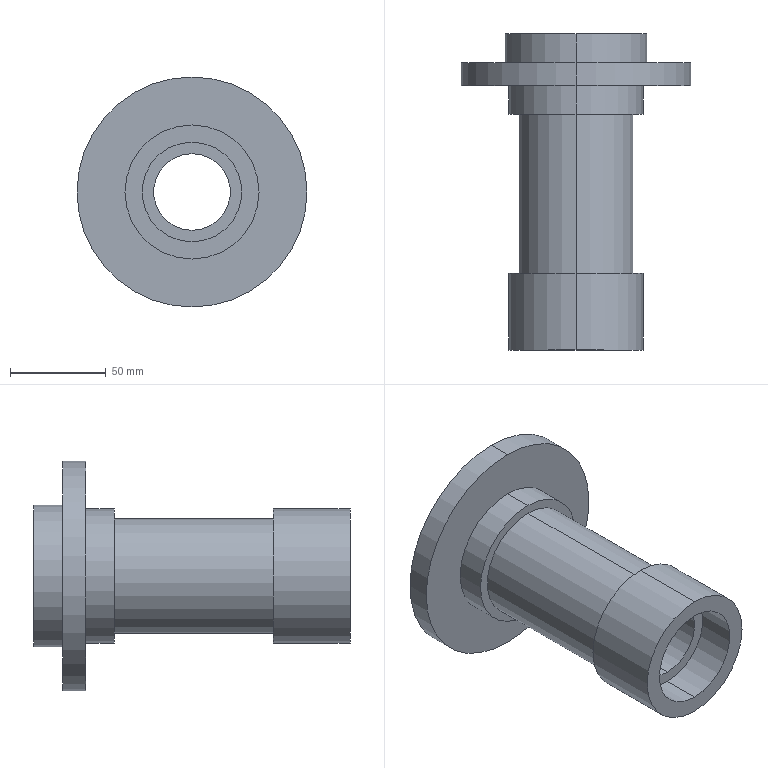Part | SolidWorks | features Revolution 1 | 1 solid | 24 faces | box 120 x 165 x 120 mm | volume 395872 mm3 | cylinder 16 | plane 8 | commonest cylinder face diameters 52 x4 70 x4 40 x2 60 x2 74 x2 120 x2
STEP:
#1=CARTESIAN_POINT('',(521.231,804.896,-470.693));
#2=VERTEX_POINT('',#1);
#3=CARTESIAN_POINT('',(521.231,804.896,-410.693));
#4=VERTEX_POINT('',#3);
#5=CARTESIAN_POINT('',(521.231,804.896,-440.693));
#6=DIRECTION('',(0.,-1.,0.));
#7=DIRECTION('',(0.,0.,-1.));
#8=AXIS2_PLACEMENT_3D('',#5,#6,#7);
#9=CIRCLE('',#8,30.);
#10=EDGE_CURVE('',#2,#4,#9,.T.);
#11=ORIENTED_EDGE('',*,*,#10,.T.);
#12=CARTESIAN_POINT('',(521.231,721.896,-410.693));
#13=VERTEX_POINT('',#12);
#14=CARTESIAN_POINT('',(521.231,846.896,-410.693));
#15=DIRECTION('',(0.,-1.,0.));
#16=VECTOR('',#15,1000.);
#17=LINE('',#14,#16);
#18=EDGE_CURVE('',#4,#13,#17,.T.);
#19=ORIENTED_EDGE('',*,*,#18,.T.);
#20=CARTESIAN_POINT('',(521.231,721.896,-470.693));
#21=VERTEX_POINT('',#20);
#22=CARTESIAN_POINT('',(521.231,721.896,-440.693));
#23=DIRECTION('',(0.,-1.,0.));
#24=DIRECTION('',(0.,0.,-1.));
#25=AXIS2_PLACEMENT_3D('',#22,#23,#24);
#26=CIRCLE('',#25,30.);
#27=EDGE_CURVE('',#21,#13,#26,.T.);
#28=ORIENTED_EDGE('',*,*,#27,.F.);
#29=CARTESIAN_POINT('',(521.231,846.896,-470.693));
#30=DIRECTION('',(0.,-1.,0.));
#31=VECTOR('',#30,1000.);
#32=LINE('',#29,#31);
#33=EDGE_CURVE('',#2,#21,#32,.T.);
#34=ORIENTED_EDGE('',*,*,#33,.F.);
#35=EDGE_LOOP('',(#11,#19,#28,#34));
#36=FACE_OUTER_BOUND('',#35,.T.);
#37=CARTESIAN_POINT('',(521.231,846.896,-440.693));
#38=DIRECTION('',(0.,-1.,0.));
#39=DIRECTION('',(0.,0.,-1.));
#40=AXIS2_PLACEMENT_3D('',#37,#38,#39);
#41=CYLINDRICAL_SURFACE('',#40,30.);
#42=ADVANCED_FACE('',(#36),#41,.T.);
#43=CARTESIAN_POINT('',(521.231,819.896,-475.693));
#44=VERTEX_POINT('',#43);
#45=CARTESIAN_POINT('',(521.231,819.896,-405.693));
#46=VERTEX_POINT('',#45);
#47=CARTESIAN_POINT('',(521.231,819.896,-440.693));
#48=DIRECTION('',(0.,-1.,0.));
#49=DIRECTION('',(0.,0.,-1.));
#50=AXIS2_PLACEMENT_3D('',#47,#48,#49);
#51=CIRCLE('',#50,35.);
#52=EDGE_CURVE('',#44,#46,#51,.T.);
#53=ORIENTED_EDGE('',*,*,#52,.T.);
#54=CARTESIAN_POINT('',(521.231,804.896,-405.693));
#55=VERTEX_POINT('',#54);
#56=CARTESIAN_POINT('',(521.231,846.896,-405.693));
#57=DIRECTION('',(0.,-1.,0.));
#58=VECTOR('',#57,1000.);
#59=LINE('',#56,#58);
#60=EDGE_CURVE('',#46,#55,#59,.T.);
#61=ORIENTED_EDGE('',*,*,#60,.T.);
#62=CARTESIAN_POINT('',(521.231,804.896,-475.693));
#63=VERTEX_POINT('',#62);
#64=CARTESIAN_POINT('',(521.231,804.896,-440.693));
#65=DIRECTION('',(0.,-1.,0.));
#66=DIRECTION('',(0.,0.,-1.));
#67=AXIS2_PLACEMENT_3D('',#64,#65,#66);
#68=CIRCLE('',#67,35.);
#69=EDGE_CURVE('',#63,#55,#68,.T.);
#70=ORIENTED_EDGE('',*,*,#69,.F.);
#71=CARTESIAN_POINT('',(521.231,846.896,-475.693));
#72=DIRECTION('',(0.,-1.,0.));
#73=VECTOR('',#72,1000.);
#74=LINE('',#71,#73);
#75=EDGE_CURVE('',#44,#63,#74,.T.);
#76=ORIENTED_EDGE('',*,*,#75,.F.);
#77=EDGE_LOOP('',(#53,#61,#70,#76));
#78=FACE_OUTER_BOUND('',#77,.T.);
#79=CARTESIAN_POINT('',(521.231,846.896,-440.693));
#80=DIRECTION('',(0.,-1.,0.));
#81=DIRECTION('',(0.,0.,-1.));
#82=AXIS2_PLACEMENT_3D('',#79,#80,#81);
#83=CYLINDRICAL_SURFACE('',#82,35.);
#84=ADVANCED_FACE('',(#78),#83,.T.);
#85=CARTESIAN_POINT('',(521.231,831.896,-500.693));
#86=VERTEX_POINT('',#85);
#87=CARTESIAN_POINT('',(521.231,831.896,-380.693));
#88=VERTEX_POINT('',#87);
#89=CARTESIAN_POINT('',(521.231,831.896,-440.693));
#90=DIRECTION('',(0.,-1.,0.));
#91=DIRECTION('',(0.,0.,-1.));
#92=AXIS2_PLACEMENT_3D('',#89,#90,#91);
#93=CIRCLE('',#92,60.);
#94=EDGE_CURVE('',#86,#88,#93,.T.);
#95=ORIENTED_EDGE('',*,*,#94,.T.);
#96=CARTESIAN_POINT('',(521.231,819.896,-380.693));
#97=VERTEX_POINT('',#96);
#98=CARTESIAN_POINT('',(521.231,846.896,-380.693));
#99=DIRECTION('',(0.,-1.,0.));
#100=VECTOR('',#99,1000.);
#101=LINE('',#98,#100);
#102=EDGE_CURVE('',#88,#97,#101,.T.);
#103=ORIENTED_EDGE('',*,*,#102,.T.);
#104=CARTESIAN_POINT('',(521.231,819.896,-500.693));
#105=VERTEX_POINT('',#104);
#106=CARTESIAN_POINT('',(521.231,819.896,-440.693));
#107=DIRECTION('',(0.,-1.,0.));
#108=DIRECTION('',(0.,0.,-1.));
#109=AXIS2_PLACEMENT_3D('',#106,#107,#108);
#110=CIRCLE('',#109,60.);
#111=EDGE_CURVE('',#105,#97,#110,.T.);
#112=ORIENTED_EDGE('',*,*,#111,.F.);
#113=CARTESIAN_POINT('',(521.231,846.896,-500.693));
#114=DIRECTION('',(0.,-1.,0.));
#115=VECTOR('',#114,1000.);
#116=LINE('',#113,#115);
#117=EDGE_CURVE('',#86,#105,#116,.T.);
#118=ORIENTED_EDGE('',*,*,#117,.F.);
#119=EDGE_LOOP('',(#95,#103,#112,#118));
#120=FACE_OUTER_BOUND('',#119,.T.);
#121=CARTESIAN_POINT('',(521.231,846.896,-440.693));
#122=DIRECTION('',(0.,-1.,0.));
#123=DIRECTION('',(0.,0.,-1.));
#124=AXIS2_PLACEMENT_3D('',#121,#122,#123);
#125=CYLINDRICAL_SURFACE('',#124,60.);
#126=ADVANCED_FACE('',(#120),#125,.T.);
#127=CARTESIAN_POINT('',(521.231,846.896,-477.693));
#128=VERTEX_POINT('',#127);
#129=CARTESIAN_POINT('',(521.231,846.896,-403.693));
#130=VERTEX_POINT('',#129);
#131=CARTESIAN_POINT('',(521.231,846.896,-440.693));
#132=DIRECTION('',(0.,-1.,0.));
#133=DIRECTION('',(0.,0.,-1.));
#134=AXIS2_PLACEMENT_3D('',#131,#132,#133);
#135=CIRCLE('',#134,37.);
#136=EDGE_CURVE('',#128,#130,#135,.T.);
#137=ORIENTED_EDGE('',*,*,#136,.T.);
#138=CARTESIAN_POINT('',(521.231,831.896,-403.693));
#139=VERTEX_POINT('',#138);
#140=CARTESIAN_POINT('',(521.231,846.896,-403.693));
#141=DIRECTION('',(0.,-1.,0.));
#142=VECTOR('',#141,1000.);
#143=LINE('',#140,#142);
#144=EDGE_CURVE('',#130,#139,#143,.T.);
#145=ORIENTED_EDGE('',*,*,#144,.T.);
#146=CARTESIAN_POINT('',(521.231,831.896,-477.693));
#147=VERTEX_POINT('',#146);
#148=CARTESIAN_POINT('',(521.231,831.896,-440.693));
#149=DIRECTION('',(0.,-1.,0.));
#150=DIRECTION('',(0.,0.,-1.));
#151=AXIS2_PLACEMENT_3D('',#148,#149,#150);
#152=CIRCLE('',#151,37.);
#153=EDGE_CURVE('',#147,#139,#152,.T.);
#154=ORIENTED_EDGE('',*,*,#153,.F.);
#155=CARTESIAN_POINT('',(521.231,846.896,-477.693));
#156=DIRECTION('',(0.,-1.,0.));
#157=VECTOR('',#156,1000.);
#158=LINE('',#155,#157);
#159=EDGE_CURVE('',#128,#147,#158,.T.);
#160=ORIENTED_EDGE('',*,*,#159,.F.);
#161=EDGE_LOOP('',(#137,#145,#154,#160));
#162=FACE_OUTER_BOUND('',#161,.T.);
#163=CARTESIAN_POINT('',(521.231,846.896,-440.693));
#164=DIRECTION('',(0.,-1.,0.));
#165=DIRECTION('',(0.,0.,-1.));
#166=AXIS2_PLACEMENT_3D('',#163,#164,#165);
#167=CYLINDRICAL_SURFACE('',#166,37.);
#168=ADVANCED_FACE('',(#162),#167,.T.);
#169=CARTESIAN_POINT('',(521.231,846.896,-414.693));
#170=VERTEX_POINT('',#169);
#171=CARTESIAN_POINT('',(521.231,846.896,-466.693));
#172=VERTEX_POINT('',#171);
#173=CARTESIAN_POINT('',(521.231,846.896,-440.693));
#174=DIRECTION('',(0.,-1.,0.));
#175=DIRECTION('',(0.,0.,-1.));
#176=AXIS2_PLACEMENT_3D('',#173,#174,#175);
#177=CIRCLE('',#176,26.);
#178=EDGE_CURVE('',#170,#172,#177,.T.);
#179=ORIENTED_EDGE('',*,*,#178,.F.);
#180=CARTESIAN_POINT('',(521.231,816.896,-414.693));
#181=VERTEX_POINT('',#180);
#182=CARTESIAN_POINT('',(521.231,846.896,-414.693));
#183=DIRECTION('',(0.,-1.,0.));
#184=VECTOR('',#183,1000.);
#185=LINE('',#182,#184);
#186=EDGE_CURVE('',#170,#181,#185,.T.);
#187=ORIENTED_EDGE('',*,*,#186,.T.);
#188=CARTESIAN_POINT('',(521.231,816.896,-466.693));
#189=VERTEX_POINT('',#188);
#190=CARTESIAN_POINT('',(521.231,816.896,-440.693));
#191=DIRECTION('',(0.,-1.,0.));
#192=DIRECTION('',(0.,0.,-1.));
#193=AXIS2_PLACEMENT_3D('',#190,#191,#192);
#194=CIRCLE('',#193,26.);
#195=EDGE_CURVE('',#181,#189,#194,.T.);
#196=ORIENTED_EDGE('',*,*,#195,.T.);
#197=CARTESIAN_POINT('',(521.231,846.896,-466.693));
#198=DIRECTION('',(0.,-1.,0.));
#199=VECTOR('',#198,1000.);
#200=LINE('',#197,#199);
#201=EDGE_CURVE('',#172,#189,#200,.T.);
#202=ORIENTED_EDGE('',*,*,#201,.F.);
#203=EDGE_LOOP('',(#179,#187,#196,#202));
#204=FACE_OUTER_BOUND('',#203,.T.);
#205=CARTESIAN_POINT('',(521.231,846.896,-440.693));
#206=DIRECTION('',(0.,-1.,0.));
#207=DIRECTION('',(0.,0.,-1.));
#208=AXIS2_PLACEMENT_3D('',#205,#206,#207);
#209=CYLINDRICAL_SURFACE('',#208,26.);
#210=ADVANCED_FACE('',(#204),#209,.F.);
#211=CARTESIAN_POINT('',(521.231,816.896,-420.693));
#212=VERTEX_POINT('',#211);
#213=CARTESIAN_POINT('',(521.231,816.896,-460.693));
#214=VERTEX_POINT('',#213);
#215=CARTESIAN_POINT('',(521.231,816.896,-440.693));
#216=DIRECTION('',(0.,-1.,0.));
#217=DIRECTION('',(0.,0.,-1.));
#218=AXIS2_PLACEMENT_3D('',#215,#216,#217);
#219=CIRCLE('',#218,20.);
#220=EDGE_CURVE('',#212,#214,#219,.T.);
#221=ORIENTED_EDGE('',*,*,#220,.F.);
#222=CARTESIAN_POINT('',(521.231,701.896,-420.693));
#223=VERTEX_POINT('',#222);
#224=CARTESIAN_POINT('',(521.231,846.896,-420.693));
#225=DIRECTION('',(0.,-1.,0.));
#226=VECTOR('',#225,1000.);
#227=LINE('',#224,#226);
#228=EDGE_CURVE('',#212,#223,#227,.T.);
#229=ORIENTED_EDGE('',*,*,#228,.T.);
#230=CARTESIAN_POINT('',(521.231,701.896,-460.693));
#231=VERTEX_POINT('',#230);
#232=CARTESIAN_POINT('',(521.231,701.896,-440.693));
#233=DIRECTION('',(0.,-1.,0.));
#234=DIRECTION('',(0.,0.,-1.));
#235=AXIS2_PLACEMENT_3D('',#232,#233,#234);
#236=CIRCLE('',#235,20.);
#237=EDGE_CURVE('',#223,#231,#236,.T.);
#238=ORIENTED_EDGE('',*,*,#237,.T.);
#239=CARTESIAN_POINT('',(521.231,846.896,-460.693));
#240=DIRECTION('',(0.,-1.,0.));
#241=VECTOR('',#240,1000.);
#242=LINE('',#239,#241);
#243=EDGE_CURVE('',#214,#231,#242,.T.);
#244=ORIENTED_EDGE('',*,*,#243,.F.);
#245=EDGE_LOOP('',(#221,#229,#238,#244));
#246=FACE_OUTER_BOUND('',#245,.T.);
#247=CARTESIAN_POINT('',(521.231,846.896,-440.693));
#248=DIRECTION('',(0.,-1.,0.));
#249=DIRECTION('',(0.,0.,-1.));
#250=AXIS2_PLACEMENT_3D('',#247,#248,#249);
#251=CYLINDRICAL_SURFACE('',#250,20.);
#252=ADVANCED_FACE('',(#246),#251,.F.);
#253=CARTESIAN_POINT('',(521.231,701.896,-414.693));
#254=VERTEX_POINT('',#253);
#255=CARTESIAN_POINT('',(521.231,701.896,-466.693));
#256=VERTEX_POINT('',#255);
#257=CARTESIAN_POINT('',(521.231,701.896,-440.693));
#258=DIRECTION('',(0.,-1.,0.));
#259=DIRECTION('',(0.,0.,-1.));
#260=AXIS2_PLACEMENT_3D('',#257,#258,#259);
#261=CIRCLE('',#260,26.);
#262=EDGE_CURVE('',#254,#256,#261,.T.);
#263=ORIENTED_EDGE('',*,*,#262,.F.);
#264=CARTESIAN_POINT('',(521.231,681.896,-414.693));
#265=VERTEX_POINT('',#264);
#266=CARTESIAN_POINT('',(521.231,846.896,-414.693));
#267=DIRECTION('',(0.,-1.,0.));
#268=VECTOR('',#267,1000.);
#269=LINE('',#266,#268);
#270=EDGE_CURVE('',#254,#265,#269,.T.);
#271=ORIENTED_EDGE('',*,*,#270,.T.);
#272=CARTESIAN_POINT('',(521.231,681.896,-466.693));
#273=VERTEX_POINT('',#272);
#274=CARTESIAN_POINT('',(521.231,681.896,-440.693));
#275=DIRECTION('',(0.,-1.,0.));
#276=DIRECTION('',(0.,0.,-1.));
#277=AXIS2_PLACEMENT_3D('',#274,#275,#276);
#278=CIRCLE('',#277,26.);
#279=EDGE_CURVE('',#265,#273,#278,.T.);
#280=ORIENTED_EDGE('',*,*,#279,.T.);
#281=CARTESIAN_POINT('',(521.231,846.896,-466.693));
#282=DIRECTION('',(0.,-1.,0.));
#283=VECTOR('',#282,1000.);
#284=LINE('',#281,#283);
#285=EDGE_CURVE('',#256,#273,#284,.T.);
#286=ORIENTED_EDGE('',*,*,#285,.F.);
#287=EDGE_LOOP('',(#263,#271,#280,#286));
#288=FACE_OUTER_BOUND('',#287,.T.);
#289=CARTESIAN_POINT('',(521.231,846.896,-440.693));
#290=DIRECTION('',(0.,-1.,0.));
#291=DIRECTION('',(0.,0.,-1.));
#292=AXIS2_PLACEMENT_3D('',#289,#290,#291);
#293=CYLINDRICAL_SURFACE('',#292,26.);
#294=ADVANCED_FACE('',(#288),#293,.F.);
#295=CARTESIAN_POINT('',(521.231,721.896,-475.693));
#296=VERTEX_POINT('',#295);
#297=CARTESIAN_POINT('',(521.231,721.896,-405.693));
#298=VERTEX_POINT('',#297);
#299=CARTESIAN_POINT('',(521.231,721.896,-440.693));
#300=DIRECTION('',(0.,-1.,0.));
#301=DIRECTION('',(0.,0.,-1.));
#302=AXIS2_PLACEMENT_3D('',#299,#300,#301);
#303=CIRCLE('',#302,35.);
#304=EDGE_CURVE('',#296,#298,#303,.T.);
#305=ORIENTED_EDGE('',*,*,#304,.T.);
#306=CARTESIAN_POINT('',(521.231,681.896,-405.693));
#307=VERTEX_POINT('',#306);
#308=CARTESIAN_POINT('',(521.231,846.896,-405.693));
#309=DIRECTION('',(0.,-1.,0.));
#310=VECTOR('',#309,1000.);
#311=LINE('',#308,#310);
#312=EDGE_CURVE('',#298,#307,#311,.T.);
#313=ORIENTED_EDGE('',*,*,#312,.T.);
#314=CARTESIAN_POINT('',(521.231,681.896,-475.693));
#315=VERTEX_POINT('',#314);
#316=CARTESIAN_POINT('',(521.231,681.896,-440.693));
#317=DIRECTION('',(0.,-1.,0.));
#318=DIRECTION('',(0.,0.,-1.));
#319=AXIS2_PLACEMENT_3D('',#316,#317,#318);
#320=CIRCLE('',#319,35.);
#321=EDGE_CURVE('',#315,#307,#320,.T.);
#322=ORIENTED_EDGE('',*,*,#321,.F.);
#323=CARTESIAN_POINT('',(521.231,846.896,-475.693));
#324=DIRECTION('',(0.,-1.,0.));
#325=VECTOR('',#324,1000.);
#326=LINE('',#323,#325);
#327=EDGE_CURVE('',#296,#315,#326,.T.);
#328=ORIENTED_EDGE('',*,*,#327,.F.);
#329=EDGE_LOOP('',(#305,#313,#322,#328));
#330=FACE_OUTER_BOUND('',#329,.T.);
#331=CARTESIAN_POINT('',(521.231,846.896,-440.693));
#332=DIRECTION('',(0.,-1.,0.));
#333=DIRECTION('',(0.,0.,-1.));
#334=AXIS2_PLACEMENT_3D('',#331,#332,#333);
#335=CYLINDRICAL_SURFACE('',#334,35.);
#336=ADVANCED_FACE('',(#330),#335,.T.);
#337=ORIENTED_EDGE('',*,*,#27,.T.);
#338=CARTESIAN_POINT('',(521.231,721.896,-440.693));
#339=DIRECTION('',(0.,-1.,0.));
#340=DIRECTION('',(0.,0.,-1.));
#341=AXIS2_PLACEMENT_3D('',#338,#339,#340);
#342=CIRCLE('',#341,30.);
#343=EDGE_CURVE('',#13,#21,#342,.T.);
#344=ORIENTED_EDGE('',*,*,#343,.T.);
#345=EDGE_LOOP('',(#337,#344));
#346=FACE_BOUND('',#345,.T.);
#347=ORIENTED_EDGE('',*,*,#304,.F.);
#348=CARTESIAN_POINT('',(521.231,721.896,-440.693));
#349=DIRECTION('',(0.,-1.,0.));
#350=DIRECTION('',(0.,0.,-1.));
#351=AXIS2_PLACEMENT_3D('',#348,#349,#350);
#352=CIRCLE('',#351,35.);
#353=EDGE_CURVE('',#298,#296,#352,.T.);
#354=ORIENTED_EDGE('',*,*,#353,.F.);
#355=EDGE_LOOP('',(#347,#354));
#356=FACE_OUTER_BOUND('',#355,.T.);
#357=CARTESIAN_POINT('',(556.231,721.896,-440.693));
#358=DIRECTION('',(0.,1.,0.));
#359=DIRECTION('',(0.,0.,1.));
#360=AXIS2_PLACEMENT_3D('',#357,#358,#359);
#361=PLANE('',#360);
#362=ADVANCED_FACE('',(#346,#356),#361,.T.);
#363=ORIENTED_EDGE('',*,*,#312,.F.);
#364=ORIENTED_EDGE('',*,*,#353,.T.);
#365=ORIENTED_EDGE('',*,*,#327,.T.);
#366=CARTESIAN_POINT('',(521.231,681.896,-440.693));
#367=DIRECTION('',(0.,-1.,0.));
#368=DIRECTION('',(0.,0.,-1.));
#369=AXIS2_PLACEMENT_3D('',#366,#367,#368);
#370=CIRCLE('',#369,35.);
#371=EDGE_CURVE('',#307,#315,#370,.T.);
#372=ORIENTED_EDGE('',*,*,#371,.F.);
#373=EDGE_LOOP('',(#363,#364,#365,#372));
#374=FACE_OUTER_BOUND('',#373,.T.);
#375=CARTESIAN_POINT('',(521.231,846.896,-440.693));
#376=DIRECTION('',(0.,-1.,0.));
#377=DIRECTION('',(0.,0.,-1.));
#378=AXIS2_PLACEMENT_3D('',#375,#376,#377);
#379=CYLINDRICAL_SURFACE('',#378,35.);
#380=ADVANCED_FACE('',(#374),#379,.T.);
#381=ORIENTED_EDGE('',*,*,#321,.T.);
#382=ORIENTED_EDGE('',*,*,#371,.T.);
#383=EDGE_LOOP('',(#381,#382));
#384=FACE_OUTER_BOUND('',#383,.T.);
#385=CARTESIAN_POINT('',(521.231,681.896,-440.693));
#386=DIRECTION('',(0.,-1.,0.));
#387=DIRECTION('',(0.,0.,-1.));
#388=AXIS2_PLACEMENT_3D('',#385,#386,#387);
#389=CIRCLE('',#388,26.);
#390=EDGE_CURVE('',#273,#265,#389,.T.);
#391=ORIENTED_EDGE('',*,*,#390,.F.);
#392=ORIENTED_EDGE('',*,*,#279,.F.);
#393=EDGE_LOOP('',(#391,#392));
#394=FACE_BOUND('',#393,.T.);
#395=CARTESIAN_POINT('',(547.231,681.896,-440.693));
#396=DIRECTION('',(0.,-1.,0.));
#397=DIRECTION('',(0.,0.,-1.));
#398=AXIS2_PLACEMENT_3D('',#395,#396,#397);
#399=PLANE('',#398);
#400=ADVANCED_FACE('',(#384,#394),#399,.T.);
#401=ORIENTED_EDGE('',*,*,#270,.F.);
#402=CARTESIAN_POINT('',(521.231,701.896,-440.693));
#403=DIRECTION('',(0.,-1.,0.));
#404=DIRECTION('',(0.,0.,-1.));
#405=AXIS2_PLACEMENT_3D('',#402,#403,#404);
#406=CIRCLE('',#405,26.);
#407=EDGE_CURVE('',#256,#254,#406,.T.);
#408=ORIENTED_EDGE('',*,*,#407,.F.);
#409=ORIENTED_EDGE('',*,*,#285,.T.);
#410=ORIENTED_EDGE('',*,*,#390,.T.);
#411=EDGE_LOOP('',(#401,#408,#409,#410));
#412=FACE_OUTER_BOUND('',#411,.T.);
#413=CARTESIAN_POINT('',(521.231,846.896,-440.693));
#414=DIRECTION('',(0.,-1.,0.));
#415=DIRECTION('',(0.,0.,-1.));
#416=AXIS2_PLACEMENT_3D('',#413,#414,#415);
#417=CYLINDRICAL_SURFACE('',#416,26.);
#418=ADVANCED_FACE('',(#412),#417,.F.);
#419=ORIENTED_EDGE('',*,*,#407,.T.);
#420=ORIENTED_EDGE('',*,*,#262,.T.);
#421=EDGE_LOOP('',(#419,#420));
#422=FACE_OUTER_BOUND('',#421,.T.);
#423=CARTESIAN_POINT('',(521.231,701.896,-440.693));
#424=DIRECTION('',(0.,-1.,0.));
#425=DIRECTION('',(0.,0.,-1.));
#426=AXIS2_PLACEMENT_3D('',#423,#424,#425);
#427=CIRCLE('',#426,20.);
#428=EDGE_CURVE('',#231,#223,#427,.T.);
#429=ORIENTED_EDGE('',*,*,#428,.F.);
#430=ORIENTED_EDGE('',*,*,#237,.F.);
#431=EDGE_LOOP('',(#429,#430));
#432=FACE_BOUND('',#431,.T.);
#433=CARTESIAN_POINT('',(541.231,701.896,-440.693));
#434=DIRECTION('',(0.,-1.,0.));
#435=DIRECTION('',(0.,0.,-1.));
#436=AXIS2_PLACEMENT_3D('',#433,#434,#435);
#437=PLANE('',#436);
#438=ADVANCED_FACE('',(#422,#432),#437,.T.);
#439=ORIENTED_EDGE('',*,*,#228,.F.);
#440=CARTESIAN_POINT('',(521.231,816.896,-440.693));
#441=DIRECTION('',(0.,-1.,0.));
#442=DIRECTION('',(0.,0.,-1.));
#443=AXIS2_PLACEMENT_3D('',#440,#441,#442);
#444=CIRCLE('',#443,20.);
#445=EDGE_CURVE('',#214,#212,#444,.T.);
#446=ORIENTED_EDGE('',*,*,#445,.F.);
#447=ORIENTED_EDGE('',*,*,#243,.T.);
#448=ORIENTED_EDGE('',*,*,#428,.T.);
#449=EDGE_LOOP('',(#439,#446,#447,#448));
#450=FACE_OUTER_BOUND('',#449,.T.);
#451=CARTESIAN_POINT('',(521.231,846.896,-440.693));
#452=DIRECTION('',(0.,-1.,0.));
#453=DIRECTION('',(0.,0.,-1.));
#454=AXIS2_PLACEMENT_3D('',#451,#452,#453);
#455=CYLINDRICAL_SURFACE('',#454,20.);
#456=ADVANCED_FACE('',(#450),#455,.F.);
#457=ORIENTED_EDGE('',*,*,#445,.T.);
#458=ORIENTED_EDGE('',*,*,#220,.T.);
#459=EDGE_LOOP('',(#457,#458));
#460=FACE_BOUND('',#459,.T.);
#461=CARTESIAN_POINT('',(521.231,816.896,-440.693));
#462=DIRECTION('',(0.,-1.,0.));
#463=DIRECTION('',(0.,0.,-1.));
#464=AXIS2_PLACEMENT_3D('',#461,#462,#463);
#465=CIRCLE('',#464,26.);
#466=EDGE_CURVE('',#189,#181,#465,.T.);
#467=ORIENTED_EDGE('',*,*,#466,.F.);
#468=ORIENTED_EDGE('',*,*,#195,.F.);
#469=EDGE_LOOP('',(#467,#468));
#470=FACE_OUTER_BOUND('',#469,.T.);
#471=CARTESIAN_POINT('',(547.231,816.896,-440.693));
#472=DIRECTION('',(0.,1.,0.));
#473=DIRECTION('',(0.,0.,1.));
#474=AXIS2_PLACEMENT_3D('',#471,#472,#473);
#475=PLANE('',#474);
#476=ADVANCED_FACE('',(#460,#470),#475,.T.);
#477=ORIENTED_EDGE('',*,*,#186,.F.);
#478=CARTESIAN_POINT('',(521.231,846.896,-440.693));
#479=DIRECTION('',(0.,-1.,0.));
#480=DIRECTION('',(0.,0.,-1.));
#481=AXIS2_PLACEMENT_3D('',#478,#479,#480);
#482=CIRCLE('',#481,26.);
#483=EDGE_CURVE('',#172,#170,#482,.T.);
#484=ORIENTED_EDGE('',*,*,#483,.F.);
#485=ORIENTED_EDGE('',*,*,#201,.T.);
#486=ORIENTED_EDGE('',*,*,#466,.T.);
#487=EDGE_LOOP('',(#477,#484,#485,#486));
#488=FACE_OUTER_BOUND('',#487,.T.);
#489=CARTESIAN_POINT('',(521.231,846.896,-440.693));
#490=DIRECTION('',(0.,-1.,0.));
#491=DIRECTION('',(0.,0.,-1.));
#492=AXIS2_PLACEMENT_3D('',#489,#490,#491);
#493=CYLINDRICAL_SURFACE('',#492,26.);
#494=ADVANCED_FACE('',(#488),#493,.F.);
#495=ORIENTED_EDGE('',*,*,#483,.T.);
#496=ORIENTED_EDGE('',*,*,#178,.T.);
#497=EDGE_LOOP('',(#495,#496));
#498=FACE_BOUND('',#497,.T.);
#499=ORIENTED_EDGE('',*,*,#136,.F.);
#500=CARTESIAN_POINT('',(521.231,846.896,-440.693));
#501=DIRECTION('',(0.,-1.,0.));
#502=DIRECTION('',(0.,0.,-1.));
#503=AXIS2_PLACEMENT_3D('',#500,#501,#502);
#504=CIRCLE('',#503,37.);
#505=EDGE_CURVE('',#130,#128,#504,.T.);
#506=ORIENTED_EDGE('',*,*,#505,.F.);
#507=EDGE_LOOP('',(#499,#506));
#508=FACE_OUTER_BOUND('',#507,.T.);
#509=CARTESIAN_POINT('',(558.231,846.896,-440.693));
#510=DIRECTION('',(0.,1.,0.));
#511=DIRECTION('',(0.,0.,1.));
#512=AXIS2_PLACEMENT_3D('',#509,#510,#511);
#513=PLANE('',#512);
#514=ADVANCED_FACE('',(#498,#508),#513,.T.);
#515=ORIENTED_EDGE('',*,*,#144,.F.);
#516=ORIENTED_EDGE('',*,*,#505,.T.);
#517=ORIENTED_EDGE('',*,*,#159,.T.);
#518=CARTESIAN_POINT('',(521.231,831.896,-440.693));
#519=DIRECTION('',(0.,-1.,0.));
#520=DIRECTION('',(0.,0.,-1.));
#521=AXIS2_PLACEMENT_3D('',#518,#519,#520);
#522=CIRCLE('',#521,37.);
#523=EDGE_CURVE('',#139,#147,#522,.T.);
#524=ORIENTED_EDGE('',*,*,#523,.F.);
#525=EDGE_LOOP('',(#515,#516,#517,#524));
#526=FACE_OUTER_BOUND('',#525,.T.);
#527=CARTESIAN_POINT('',(521.231,846.896,-440.693));
#528=DIRECTION('',(0.,-1.,0.));
#529=DIRECTION('',(0.,0.,-1.));
#530=AXIS2_PLACEMENT_3D('',#527,#528,#529);
#531=CYLINDRICAL_SURFACE('',#530,37.);
#532=ADVANCED_FACE('',(#526),#531,.T.);
#533=ORIENTED_EDGE('',*,*,#153,.T.);
#534=ORIENTED_EDGE('',*,*,#523,.T.);
#535=EDGE_LOOP('',(#533,#534));
#536=FACE_BOUND('',#535,.T.);
#537=ORIENTED_EDGE('',*,*,#94,.F.);
#538=CARTESIAN_POINT('',(521.231,831.896,-440.693));
#539=DIRECTION('',(0.,-1.,0.));
#540=DIRECTION('',(0.,0.,-1.));
#541=AXIS2_PLACEMENT_3D('',#538,#539,#540);
#542=CIRCLE('',#541,60.);
#543=EDGE_CURVE('',#88,#86,#542,.T.);
#544=ORIENTED_EDGE('',*,*,#543,.F.);
#545=EDGE_LOOP('',(#537,#544));
#546=FACE_OUTER_BOUND('',#545,.T.);
#547=CARTESIAN_POINT('',(581.231,831.896,-440.693));
#548=DIRECTION('',(0.,1.,0.));
#549=DIRECTION('',(0.,0.,1.));
#550=AXIS2_PLACEMENT_3D('',#547,#548,#549);
#551=PLANE('',#550);
#552=ADVANCED_FACE('',(#536,#546),#551,.T.);
#553=ORIENTED_EDGE('',*,*,#102,.F.);
#554=ORIENTED_EDGE('',*,*,#543,.T.);
#555=ORIENTED_EDGE('',*,*,#117,.T.);
#556=CARTESIAN_POINT('',(521.231,819.896,-440.693));
#557=DIRECTION('',(0.,-1.,0.));
#558=DIRECTION('',(0.,0.,-1.));
#559=AXIS2_PLACEMENT_3D('',#556,#557,#558);
#560=CIRCLE('',#559,60.);
#561=EDGE_CURVE('',#97,#105,#560,.T.);
#562=ORIENTED_EDGE('',*,*,#561,.F.);
#563=EDGE_LOOP('',(#553,#554,#555,#562));
#564=FACE_OUTER_BOUND('',#563,.T.);
#565=CARTESIAN_POINT('',(521.231,846.896,-440.693));
#566=DIRECTION('',(0.,-1.,0.));
#567=DIRECTION('',(0.,0.,-1.));
#568=AXIS2_PLACEMENT_3D('',#565,#566,#567);
#569=CYLINDRICAL_SURFACE('',#568,60.);
#570=ADVANCED_FACE('',(#564),#569,.T.);
#571=ORIENTED_EDGE('',*,*,#111,.T.);
#572=ORIENTED_EDGE('',*,*,#561,.T.);
#573=EDGE_LOOP('',(#571,#572));
#574=FACE_OUTER_BOUND('',#573,.T.);
#575=ORIENTED_EDGE('',*,*,#52,.F.);
#576=CARTESIAN_POINT('',(521.231,819.896,-440.693));
#577=DIRECTION('',(0.,-1.,0.));
#578=DIRECTION('',(0.,0.,-1.));
#579=AXIS2_PLACEMENT_3D('',#576,#577,#578);
#580=CIRCLE('',#579,35.);
#581=EDGE_CURVE('',#46,#44,#580,.T.);
#582=ORIENTED_EDGE('',*,*,#581,.F.);
#583=EDGE_LOOP('',(#575,#582));
#584=FACE_BOUND('',#583,.T.);
#585=CARTESIAN_POINT('',(556.231,819.896,-440.693));
#586=DIRECTION('',(0.,-1.,0.));
#587=DIRECTION('',(0.,0.,-1.));
#588=AXIS2_PLACEMENT_3D('',#585,#586,#587);
#589=PLANE('',#588);
#590=ADVANCED_FACE('',(#574,#584),#589,.T.);
#591=ORIENTED_EDGE('',*,*,#60,.F.);
#592=ORIENTED_EDGE('',*,*,#581,.T.);
#593=ORIENTED_EDGE('',*,*,#75,.T.);
#594=CARTESIAN_POINT('',(521.231,804.896,-440.693));
#595=DIRECTION('',(0.,-1.,0.));
#596=DIRECTION('',(0.,0.,-1.));
#597=AXIS2_PLACEMENT_3D('',#594,#595,#596);
#598=CIRCLE('',#597,35.);
#599=EDGE_CURVE('',#55,#63,#598,.T.);
#600=ORIENTED_EDGE('',*,*,#599,.F.);
#601=EDGE_LOOP('',(#591,#592,#593,#600));
#602=FACE_OUTER_BOUND('',#601,.T.);
#603=CARTESIAN_POINT('',(521.231,846.896,-440.693));
#604=DIRECTION('',(0.,-1.,0.));
#605=DIRECTION('',(0.,0.,-1.));
#606=AXIS2_PLACEMENT_3D('',#603,#604,#605);
#607=CYLINDRICAL_SURFACE('',#606,35.);
#608=ADVANCED_FACE('',(#602),#607,.T.);
#609=ORIENTED_EDGE('',*,*,#69,.T.);
#610=ORIENTED_EDGE('',*,*,#599,.T.);
#611=EDGE_LOOP('',(#609,#610));
#612=FACE_OUTER_BOUND('',#611,.T.);
#613=ORIENTED_EDGE('',*,*,#10,.F.);
#614=CARTESIAN_POINT('',(521.231,804.896,-440.693));
#615=DIRECTION('',(0.,-1.,0.));
#616=DIRECTION('',(0.,0.,-1.));
#617=AXIS2_PLACEMENT_3D('',#614,#615,#616);
#618=CIRCLE('',#617,30.);
#619=EDGE_CURVE('',#4,#2,#618,.T.);
#620=ORIENTED_EDGE('',*,*,#619,.F.);
#621=EDGE_LOOP('',(#613,#620));
#622=FACE_BOUND('',#621,.T.);
#623=CARTESIAN_POINT('',(551.231,804.896,-440.693));
#624=DIRECTION('',(0.,-1.,0.));
#625=DIRECTION('',(0.,0.,-1.));
#626=AXIS2_PLACEMENT_3D('',#623,#624,#625);
#627=PLANE('',#626);
#628=ADVANCED_FACE('',(#612,#622),#627,.T.);
#629=ORIENTED_EDGE('',*,*,#18,.F.);
#630=ORIENTED_EDGE('',*,*,#619,.T.);
#631=ORIENTED_EDGE('',*,*,#33,.T.);
#632=ORIENTED_EDGE('',*,*,#343,.F.);
#633=EDGE_LOOP('',(#629,#630,#631,#632));
#634=FACE_OUTER_BOUND('',#633,.T.);
#635=CARTESIAN_POINT('',(521.231,846.896,-440.693));
#636=DIRECTION('',(0.,-1.,0.));
#637=DIRECTION('',(0.,0.,-1.));
#638=AXIS2_PLACEMENT_3D('',#635,#636,#637);
#639=CYLINDRICAL_SURFACE('',#638,30.);
#640=ADVANCED_FACE('',(#634),#639,.T.);
#641=CLOSED_SHELL('',(#42,#84,#126,#168,#210,#252,#294,#336,#362,#380,#400,#418,#438,#456,#476,#494,#514,#532,#552,#570,#590,#608,#628,#640));
#642=MANIFOLD_SOLID_BREP('',#641);
#643=CARTESIAN_POINT('',(0.,0.,0.));
#644=DIRECTION('',(0.,0.,1.));
#645=DIRECTION('',(1.,0.,0.));
#646=AXIS2_PLACEMENT_3D('',#643,#644,#645);
#647=(LENGTH_UNIT()NAMED_UNIT(*)SI_UNIT(.MILLI.,.METRE.));
#648=UNCERTAINTY_MEASURE_WITH_UNIT(LENGTH_MEASURE(0.00001),#647,'','');
#649=(NAMED_UNIT(*)PLANE_ANGLE_UNIT()SI_UNIT($,.RADIAN.));
#650=(NAMED_UNIT(*)SI_UNIT($,.STERADIAN.)SOLID_ANGLE_UNIT());
#651=(GEOMETRIC_REPRESENTATION_CONTEXT(3)GLOBAL_UNCERTAINTY_ASSIGNED_CONTEXT((#648))GLOBAL_UNIT_ASSIGNED_CONTEXT((#647,#649,#650))REPRESENTATION_CONTEXT('',''));
#652=ADVANCED_BREP_SHAPE_REPRESENTATION('',(#642,#646),#651);